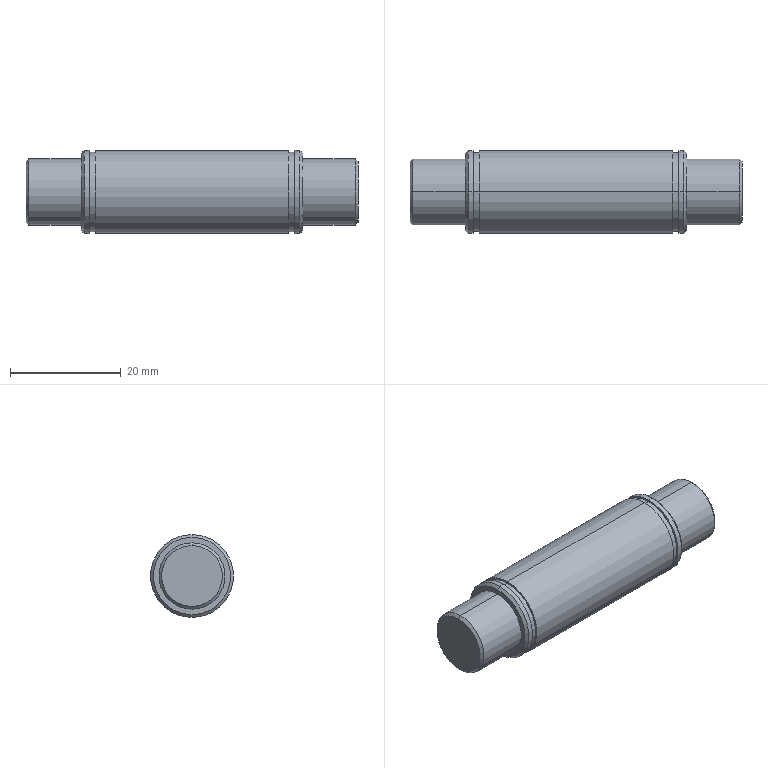Part | SolidWorks | features MirrorPattern 2, Chamfer 1, Extrusion 1, ICE 1, RevCut 1 | 1 solid | 30 faces | box 60 x 15 x 15 mm | volume 9274 mm3 | cylinder 14 | cone 8 | plane 8 | commonest cylinder face diameters 15 x6 12 x4 14.3 x4
STEP:
#1=CARTESIAN_POINT('',(19.5,0.,7.5));
#2=VERTEX_POINT('',#1);
#3=CARTESIAN_POINT('',(19.5,0.,-7.5));
#4=VERTEX_POINT('',#3);
#5=CARTESIAN_POINT('',(19.5,0.,0.));
#6=DIRECTION('',(-1.,0.,0.));
#7=DIRECTION('',(0.,0.,-1.));
#8=AXIS2_PLACEMENT_3D('',#5,#6,#7);
#9=CIRCLE('',#8,7.5);
#10=EDGE_CURVE('',#2,#4,#9,.T.);
#11=ORIENTED_EDGE('',*,*,#10,.T.);
#12=CARTESIAN_POINT('',(18.6,0.,-7.5));
#13=VERTEX_POINT('',#12);
#14=CARTESIAN_POINT('',(30.,0.,-7.5));
#15=DIRECTION('',(-1.,0.,0.));
#16=VECTOR('',#15,1000.);
#17=LINE('',#14,#16);
#18=EDGE_CURVE('',#4,#13,#17,.T.);
#19=ORIENTED_EDGE('',*,*,#18,.T.);
#20=CARTESIAN_POINT('',(18.6,0.,7.5));
#21=VERTEX_POINT('',#20);
#22=CARTESIAN_POINT('',(18.6,0.,0.));
#23=DIRECTION('',(-1.,0.,0.));
#24=DIRECTION('',(0.,0.,1.));
#25=AXIS2_PLACEMENT_3D('',#22,#23,#24);
#26=CIRCLE('',#25,7.5);
#27=EDGE_CURVE('',#21,#13,#26,.T.);
#28=ORIENTED_EDGE('',*,*,#27,.F.);
#29=CARTESIAN_POINT('',(30.,0.,7.5));
#30=DIRECTION('',(-1.,0.,0.));
#31=VECTOR('',#30,1000.);
#32=LINE('',#29,#31);
#33=EDGE_CURVE('',#2,#21,#32,.T.);
#34=ORIENTED_EDGE('',*,*,#33,.F.);
#35=EDGE_LOOP('',(#11,#19,#28,#34));
#36=FACE_OUTER_BOUND('',#35,.T.);
#37=CARTESIAN_POINT('',(30.,0.,0.));
#38=DIRECTION('',(-1.,0.,0.));
#39=DIRECTION('',(0.,0.,1.));
#40=AXIS2_PLACEMENT_3D('',#37,#38,#39);
#41=CYLINDRICAL_SURFACE('',#40,7.5);
#42=ADVANCED_FACE('',(#36),#41,.T.);
#43=CARTESIAN_POINT('',(20.,0.,-7.));
#44=VERTEX_POINT('',#43);
#45=CARTESIAN_POINT('',(20.,0.,7.));
#46=VERTEX_POINT('',#45);
#47=CARTESIAN_POINT('',(20.,0.,0.));
#48=DIRECTION('',(1.,0.,0.));
#49=DIRECTION('',(0.,0.,-1.));
#50=AXIS2_PLACEMENT_3D('',#47,#48,#49);
#51=CIRCLE('',#50,7.);
#52=EDGE_CURVE('',#44,#46,#51,.T.);
#53=ORIENTED_EDGE('',*,*,#52,.F.);
#54=CARTESIAN_POINT('',(20.,0.,-7.));
#55=DIRECTION('',(-0.7071,0.,-0.7071));
#56=VECTOR('',#55,1000.);
#57=LINE('',#54,#56);
#58=EDGE_CURVE('',#44,#4,#57,.T.);
#59=ORIENTED_EDGE('',*,*,#58,.T.);
#60=ORIENTED_EDGE('',*,*,#10,.F.);
#61=CARTESIAN_POINT('',(20.,0.,7.));
#62=DIRECTION('',(-0.7071,0.,0.7071));
#63=VECTOR('',#62,1000.);
#64=LINE('',#61,#63);
#65=EDGE_CURVE('',#46,#2,#64,.T.);
#66=ORIENTED_EDGE('',*,*,#65,.F.);
#67=EDGE_LOOP('',(#53,#59,#60,#66));
#68=FACE_OUTER_BOUND('',#67,.T.);
#69=CARTESIAN_POINT('',(20.,0.,0.));
#70=DIRECTION('',(-1.,0.,0.));
#71=DIRECTION('',(0.,0.,1.));
#72=AXIS2_PLACEMENT_3D('',#69,#70,#71);
#73=CONICAL_SURFACE('',#72,7.,0.7854);
#74=ADVANCED_FACE('',(#68),#73,.T.);
#75=CARTESIAN_POINT('',(20.,0.,-6.));
#76=VERTEX_POINT('',#75);
#77=CARTESIAN_POINT('',(20.,0.,6.));
#78=VERTEX_POINT('',#77);
#79=CARTESIAN_POINT('',(20.,0.,0.));
#80=DIRECTION('',(1.,0.,0.));
#81=DIRECTION('',(0.,0.,-1.));
#82=AXIS2_PLACEMENT_3D('',#79,#80,#81);
#83=CIRCLE('',#82,6.);
#84=EDGE_CURVE('',#76,#78,#83,.T.);
#85=ORIENTED_EDGE('',*,*,#84,.T.);
#86=CARTESIAN_POINT('',(29.5,0.,6.));
#87=VERTEX_POINT('',#86);
#88=CARTESIAN_POINT('',(20.,0.,6.));
#89=DIRECTION('',(1.,0.,0.));
#90=VECTOR('',#89,1000.);
#91=LINE('',#88,#90);
#92=EDGE_CURVE('',#78,#87,#91,.T.);
#93=ORIENTED_EDGE('',*,*,#92,.T.);
#94=CARTESIAN_POINT('',(29.5,0.,-6.));
#95=VERTEX_POINT('',#94);
#96=CARTESIAN_POINT('',(29.5,0.,0.));
#97=DIRECTION('',(-1.,0.,0.));
#98=DIRECTION('',(0.,0.,-1.));
#99=AXIS2_PLACEMENT_3D('',#96,#97,#98);
#100=CIRCLE('',#99,6.);
#101=EDGE_CURVE('',#87,#95,#100,.T.);
#102=ORIENTED_EDGE('',*,*,#101,.T.);
#103=CARTESIAN_POINT('',(20.,0.,-6.));
#104=DIRECTION('',(1.,0.,0.));
#105=VECTOR('',#104,1000.);
#106=LINE('',#103,#105);
#107=EDGE_CURVE('',#76,#95,#106,.T.);
#108=ORIENTED_EDGE('',*,*,#107,.F.);
#109=EDGE_LOOP('',(#85,#93,#102,#108));
#110=FACE_OUTER_BOUND('',#109,.T.);
#111=CARTESIAN_POINT('',(20.,0.,0.));
#112=DIRECTION('',(1.,0.,0.));
#113=DIRECTION('',(0.,0.,-1.));
#114=AXIS2_PLACEMENT_3D('',#111,#112,#113);
#115=CYLINDRICAL_SURFACE('',#114,6.);
#116=ADVANCED_FACE('',(#110),#115,.T.);
#117=CARTESIAN_POINT('',(30.,0.,-5.5));
#118=VERTEX_POINT('',#117);
#119=CARTESIAN_POINT('',(30.,0.,5.5));
#120=VERTEX_POINT('',#119);
#121=CARTESIAN_POINT('',(30.,0.,0.));
#122=DIRECTION('',(1.,0.,0.));
#123=DIRECTION('',(0.,0.,-1.));
#124=AXIS2_PLACEMENT_3D('',#121,#122,#123);
#125=CIRCLE('',#124,5.5);
#126=EDGE_CURVE('',#118,#120,#125,.T.);
#127=ORIENTED_EDGE('',*,*,#126,.F.);
#128=CARTESIAN_POINT('',(30.,0.,-5.5));
#129=DIRECTION('',(-0.7071,0.,-0.7071));
#130=VECTOR('',#129,1000.);
#131=LINE('',#128,#130);
#132=EDGE_CURVE('',#118,#95,#131,.T.);
#133=ORIENTED_EDGE('',*,*,#132,.T.);
#134=ORIENTED_EDGE('',*,*,#101,.F.);
#135=CARTESIAN_POINT('',(30.,0.,5.5));
#136=DIRECTION('',(-0.7071,0.,0.7071));
#137=VECTOR('',#136,1000.);
#138=LINE('',#135,#137);
#139=EDGE_CURVE('',#120,#87,#138,.T.);
#140=ORIENTED_EDGE('',*,*,#139,.F.);
#141=EDGE_LOOP('',(#127,#133,#134,#140));
#142=FACE_OUTER_BOUND('',#141,.T.);
#143=CARTESIAN_POINT('',(30.,0.,0.));
#144=DIRECTION('',(-1.,0.,0.));
#145=DIRECTION('',(0.,0.,1.));
#146=AXIS2_PLACEMENT_3D('',#143,#144,#145);
#147=CONICAL_SURFACE('',#146,5.5,0.7854);
#148=ADVANCED_FACE('',(#142),#147,.T.);
#149=CARTESIAN_POINT('',(17.5,0.,-7.15));
#150=VERTEX_POINT('',#149);
#151=CARTESIAN_POINT('',(17.5,0.,7.15));
#152=VERTEX_POINT('',#151);
#153=CARTESIAN_POINT('',(17.5,0.,0.));
#154=DIRECTION('',(-1.,0.,0.));
#155=DIRECTION('',(0.,0.,1.));
#156=AXIS2_PLACEMENT_3D('',#153,#154,#155);
#157=CIRCLE('',#156,7.15);
#158=EDGE_CURVE('',#150,#152,#157,.T.);
#159=ORIENTED_EDGE('',*,*,#158,.F.);
#160=CARTESIAN_POINT('',(18.6,0.,-7.15));
#161=VERTEX_POINT('',#160);
#162=CARTESIAN_POINT('',(31.366,0.,-7.15));
#163=DIRECTION('',(1.,0.,0.));
#164=VECTOR('',#163,1000.);
#165=LINE('',#162,#164);
#166=EDGE_CURVE('',#150,#161,#165,.T.);
#167=ORIENTED_EDGE('',*,*,#166,.T.);
#168=CARTESIAN_POINT('',(18.6,0.,7.15));
#169=VERTEX_POINT('',#168);
#170=CARTESIAN_POINT('',(18.6,0.,0.));
#171=DIRECTION('',(-1.,0.,0.));
#172=DIRECTION('',(0.,0.,1.));
#173=AXIS2_PLACEMENT_3D('',#170,#171,#172);
#174=CIRCLE('',#173,7.15);
#175=EDGE_CURVE('',#161,#169,#174,.T.);
#176=ORIENTED_EDGE('',*,*,#175,.T.);
#177=CARTESIAN_POINT('',(31.366,0.,7.15));
#178=DIRECTION('',(1.,0.,0.));
#179=VECTOR('',#178,1000.);
#180=LINE('',#177,#179);
#181=EDGE_CURVE('',#152,#169,#180,.T.);
#182=ORIENTED_EDGE('',*,*,#181,.F.);
#183=EDGE_LOOP('',(#159,#167,#176,#182));
#184=FACE_OUTER_BOUND('',#183,.T.);
#185=CARTESIAN_POINT('',(31.366,0.,0.));
#186=DIRECTION('',(1.,0.,0.));
#187=DIRECTION('',(0.,0.,1.));
#188=AXIS2_PLACEMENT_3D('',#185,#186,#187);
#189=CYLINDRICAL_SURFACE('',#188,7.15);
#190=ADVANCED_FACE('',(#184),#189,.T.);
#191=CARTESIAN_POINT('',(17.5,0.,7.5));
#192=VERTEX_POINT('',#191);
#193=CARTESIAN_POINT('',(17.5,0.,-7.5));
#194=VERTEX_POINT('',#193);
#195=CARTESIAN_POINT('',(17.5,0.,0.));
#196=DIRECTION('',(-1.,0.,0.));
#197=DIRECTION('',(0.,0.,1.));
#198=AXIS2_PLACEMENT_3D('',#195,#196,#197);
#199=CIRCLE('',#198,7.5);
#200=EDGE_CURVE('',#192,#194,#199,.T.);
#201=ORIENTED_EDGE('',*,*,#200,.T.);
#202=CARTESIAN_POINT('',(-17.5,0.,-7.5));
#203=VERTEX_POINT('',#202);
#204=CARTESIAN_POINT('',(30.,0.,-7.5));
#205=DIRECTION('',(-1.,0.,0.));
#206=VECTOR('',#205,1000.);
#207=LINE('',#204,#206);
#208=EDGE_CURVE('',#194,#203,#207,.T.);
#209=ORIENTED_EDGE('',*,*,#208,.T.);
#210=CARTESIAN_POINT('',(-17.5,0.,7.5));
#211=VERTEX_POINT('',#210);
#212=CARTESIAN_POINT('',(-17.5,0.,0.));
#213=DIRECTION('',(-1.,0.,0.));
#214=DIRECTION('',(0.,0.,1.));
#215=AXIS2_PLACEMENT_3D('',#212,#213,#214);
#216=CIRCLE('',#215,7.5);
#217=EDGE_CURVE('',#211,#203,#216,.T.);
#218=ORIENTED_EDGE('',*,*,#217,.F.);
#219=CARTESIAN_POINT('',(30.,0.,7.5));
#220=DIRECTION('',(-1.,0.,0.));
#221=VECTOR('',#220,1000.);
#222=LINE('',#219,#221);
#223=EDGE_CURVE('',#192,#211,#222,.T.);
#224=ORIENTED_EDGE('',*,*,#223,.F.);
#225=EDGE_LOOP('',(#201,#209,#218,#224));
#226=FACE_OUTER_BOUND('',#225,.T.);
#227=CARTESIAN_POINT('',(30.,0.,0.));
#228=DIRECTION('',(-1.,0.,0.));
#229=DIRECTION('',(0.,0.,1.));
#230=AXIS2_PLACEMENT_3D('',#227,#228,#229);
#231=CYLINDRICAL_SURFACE('',#230,7.5);
#232=ADVANCED_FACE('',(#226),#231,.T.);
#233=CARTESIAN_POINT('',(-17.5,0.,7.15));
#234=VERTEX_POINT('',#233);
#235=CARTESIAN_POINT('',(-17.5,0.,-7.15));
#236=VERTEX_POINT('',#235);
#237=CARTESIAN_POINT('',(-17.5,0.,0.));
#238=DIRECTION('',(-1.,0.,0.));
#239=DIRECTION('',(0.,0.,1.));
#240=AXIS2_PLACEMENT_3D('',#237,#238,#239);
#241=CIRCLE('',#240,7.15);
#242=EDGE_CURVE('',#234,#236,#241,.T.);
#243=ORIENTED_EDGE('',*,*,#242,.T.);
#244=CARTESIAN_POINT('',(-18.6,0.,-7.15));
#245=VERTEX_POINT('',#244);
#246=CARTESIAN_POINT('',(-31.366,0.,-7.15));
#247=DIRECTION('',(-1.,0.,0.));
#248=VECTOR('',#247,1000.);
#249=LINE('',#246,#248);
#250=EDGE_CURVE('',#236,#245,#249,.T.);
#251=ORIENTED_EDGE('',*,*,#250,.T.);
#252=CARTESIAN_POINT('',(-18.6,0.,7.15));
#253=VERTEX_POINT('',#252);
#254=CARTESIAN_POINT('',(-18.6,0.,0.));
#255=DIRECTION('',(-1.,0.,0.));
#256=DIRECTION('',(0.,0.,1.));
#257=AXIS2_PLACEMENT_3D('',#254,#255,#256);
#258=CIRCLE('',#257,7.15);
#259=EDGE_CURVE('',#253,#245,#258,.T.);
#260=ORIENTED_EDGE('',*,*,#259,.F.);
#261=CARTESIAN_POINT('',(-31.366,0.,7.15));
#262=DIRECTION('',(-1.,0.,0.));
#263=VECTOR('',#262,1000.);
#264=LINE('',#261,#263);
#265=EDGE_CURVE('',#234,#253,#264,.T.);
#266=ORIENTED_EDGE('',*,*,#265,.F.);
#267=EDGE_LOOP('',(#243,#251,#260,#266));
#268=FACE_OUTER_BOUND('',#267,.T.);
#269=CARTESIAN_POINT('',(-31.366,0.,0.));
#270=DIRECTION('',(-1.,0.,0.));
#271=DIRECTION('',(0.,0.,1.));
#272=AXIS2_PLACEMENT_3D('',#269,#270,#271);
#273=CYLINDRICAL_SURFACE('',#272,7.15);
#274=ADVANCED_FACE('',(#268),#273,.T.);
#275=CARTESIAN_POINT('',(-30.,0.,5.5));
#276=VERTEX_POINT('',#275);
#277=CARTESIAN_POINT('',(-30.,0.,-5.5));
#278=VERTEX_POINT('',#277);
#279=CARTESIAN_POINT('',(-30.,0.,0.));
#280=DIRECTION('',(-1.,0.,0.));
#281=DIRECTION('',(0.,0.,-1.));
#282=AXIS2_PLACEMENT_3D('',#279,#280,#281);
#283=CIRCLE('',#282,5.5);
#284=EDGE_CURVE('',#276,#278,#283,.T.);
#285=ORIENTED_EDGE('',*,*,#284,.F.);
#286=CARTESIAN_POINT('',(-29.5,0.,6.));
#287=VERTEX_POINT('',#286);
#288=CARTESIAN_POINT('',(-29.5,0.,6.));
#289=DIRECTION('',(0.7071,0.,0.7071));
#290=VECTOR('',#289,1000.);
#291=LINE('',#288,#290);
#292=EDGE_CURVE('',#276,#287,#291,.T.);
#293=ORIENTED_EDGE('',*,*,#292,.T.);
#294=CARTESIAN_POINT('',(-29.5,0.,-6.));
#295=VERTEX_POINT('',#294);
#296=CARTESIAN_POINT('',(-29.5,0.,0.));
#297=DIRECTION('',(1.,0.,0.));
#298=DIRECTION('',(0.,0.,-1.));
#299=AXIS2_PLACEMENT_3D('',#296,#297,#298);
#300=CIRCLE('',#299,6.);
#301=EDGE_CURVE('',#295,#287,#300,.T.);
#302=ORIENTED_EDGE('',*,*,#301,.F.);
#303=CARTESIAN_POINT('',(-29.5,0.,-6.));
#304=DIRECTION('',(0.7071,0.,-0.7071));
#305=VECTOR('',#304,1000.);
#306=LINE('',#303,#305);
#307=EDGE_CURVE('',#278,#295,#306,.T.);
#308=ORIENTED_EDGE('',*,*,#307,.F.);
#309=EDGE_LOOP('',(#285,#293,#302,#308));
#310=FACE_OUTER_BOUND('',#309,.T.);
#311=CARTESIAN_POINT('',(-29.5,0.,0.));
#312=DIRECTION('',(1.,0.,0.));
#313=DIRECTION('',(0.,0.,-1.));
#314=AXIS2_PLACEMENT_3D('',#311,#312,#313);
#315=CONICAL_SURFACE('',#314,6.,0.7854);
#316=ADVANCED_FACE('',(#310),#315,.T.);
#317=CARTESIAN_POINT('',(-20.,0.,7.));
#318=VERTEX_POINT('',#317);
#319=CARTESIAN_POINT('',(-20.,0.,-7.));
#320=VERTEX_POINT('',#319);
#321=CARTESIAN_POINT('',(-20.,0.,0.));
#322=DIRECTION('',(-1.,0.,0.));
#323=DIRECTION('',(0.,0.,1.));
#324=AXIS2_PLACEMENT_3D('',#321,#322,#323);
#325=CIRCLE('',#324,7.);
#326=EDGE_CURVE('',#318,#320,#325,.T.);
#327=ORIENTED_EDGE('',*,*,#326,.F.);
#328=CARTESIAN_POINT('',(-19.5,0.,7.5));
#329=VERTEX_POINT('',#328);
#330=CARTESIAN_POINT('',(-20.,0.,7.));
#331=DIRECTION('',(0.7071,0.,0.7071));
#332=VECTOR('',#331,1000.);
#333=LINE('',#330,#332);
#334=EDGE_CURVE('',#318,#329,#333,.T.);
#335=ORIENTED_EDGE('',*,*,#334,.T.);
#336=CARTESIAN_POINT('',(-19.5,0.,-7.5));
#337=VERTEX_POINT('',#336);
#338=CARTESIAN_POINT('',(-19.5,0.,0.));
#339=DIRECTION('',(1.,0.,0.));
#340=DIRECTION('',(0.,0.,1.));
#341=AXIS2_PLACEMENT_3D('',#338,#339,#340);
#342=CIRCLE('',#341,7.5);
#343=EDGE_CURVE('',#337,#329,#342,.T.);
#344=ORIENTED_EDGE('',*,*,#343,.F.);
#345=CARTESIAN_POINT('',(-20.,0.,-7.));
#346=DIRECTION('',(0.7071,0.,-0.7071));
#347=VECTOR('',#346,1000.);
#348=LINE('',#345,#347);
#349=EDGE_CURVE('',#320,#337,#348,.T.);
#350=ORIENTED_EDGE('',*,*,#349,.F.);
#351=EDGE_LOOP('',(#327,#335,#344,#350));
#352=FACE_OUTER_BOUND('',#351,.T.);
#353=CARTESIAN_POINT('',(-20.,0.,0.));
#354=DIRECTION('',(1.,0.,0.));
#355=DIRECTION('',(0.,0.,-1.));
#356=AXIS2_PLACEMENT_3D('',#353,#354,#355);
#357=CONICAL_SURFACE('',#356,7.,0.7854);
#358=ADVANCED_FACE('',(#352),#357,.T.);
#359=CARTESIAN_POINT('',(-20.,0.,-6.));
#360=VERTEX_POINT('',#359);
#361=CARTESIAN_POINT('',(-20.,0.,6.));
#362=VERTEX_POINT('',#361);
#363=CARTESIAN_POINT('',(-20.,0.,0.));
#364=DIRECTION('',(1.,0.,0.));
#365=DIRECTION('',(0.,0.,-1.));
#366=AXIS2_PLACEMENT_3D('',#363,#364,#365);
#367=CIRCLE('',#366,6.);
#368=EDGE_CURVE('',#360,#362,#367,.T.);
#369=ORIENTED_EDGE('',*,*,#368,.F.);
#370=CARTESIAN_POINT('',(-20.,0.,-6.));
#371=DIRECTION('',(-1.,0.,0.));
#372=VECTOR('',#371,1000.);
#373=LINE('',#370,#372);
#374=EDGE_CURVE('',#360,#295,#373,.T.);
#375=ORIENTED_EDGE('',*,*,#374,.T.);
#376=ORIENTED_EDGE('',*,*,#301,.T.);
#377=CARTESIAN_POINT('',(-20.,0.,6.));
#378=DIRECTION('',(-1.,0.,0.));
#379=VECTOR('',#378,1000.);
#380=LINE('',#377,#379);
#381=EDGE_CURVE('',#362,#287,#380,.T.);
#382=ORIENTED_EDGE('',*,*,#381,.F.);
#383=EDGE_LOOP('',(#369,#375,#376,#382));
#384=FACE_OUTER_BOUND('',#383,.T.);
#385=CARTESIAN_POINT('',(-20.,0.,0.));
#386=DIRECTION('',(-1.,0.,0.));
#387=DIRECTION('',(0.,0.,1.));
#388=AXIS2_PLACEMENT_3D('',#385,#386,#387);
#389=CYLINDRICAL_SURFACE('',#388,6.);
#390=ADVANCED_FACE('',(#384),#389,.T.);
#391=CARTESIAN_POINT('',(-18.6,0.,7.5));
#392=VERTEX_POINT('',#391);
#393=CARTESIAN_POINT('',(-18.6,0.,-7.5));
#394=VERTEX_POINT('',#393);
#395=CARTESIAN_POINT('',(-18.6,0.,0.));
#396=DIRECTION('',(-1.,0.,0.));
#397=DIRECTION('',(0.,0.,1.));
#398=AXIS2_PLACEMENT_3D('',#395,#396,#397);
#399=CIRCLE('',#398,7.5);
#400=EDGE_CURVE('',#392,#394,#399,.T.);
#401=ORIENTED_EDGE('',*,*,#400,.T.);
#402=CARTESIAN_POINT('',(30.,0.,-7.5));
#403=DIRECTION('',(-1.,0.,0.));
#404=VECTOR('',#403,1000.);
#405=LINE('',#402,#404);
#406=EDGE_CURVE('',#394,#337,#405,.T.);
#407=ORIENTED_EDGE('',*,*,#406,.T.);
#408=ORIENTED_EDGE('',*,*,#343,.T.);
#409=CARTESIAN_POINT('',(30.,0.,7.5));
#410=DIRECTION('',(-1.,0.,0.));
#411=VECTOR('',#410,1000.);
#412=LINE('',#409,#411);
#413=EDGE_CURVE('',#392,#329,#412,.T.);
#414=ORIENTED_EDGE('',*,*,#413,.F.);
#415=EDGE_LOOP('',(#401,#407,#408,#414));
#416=FACE_OUTER_BOUND('',#415,.T.);
#417=CARTESIAN_POINT('',(30.,0.,0.));
#418=DIRECTION('',(-1.,0.,0.));
#419=DIRECTION('',(0.,0.,1.));
#420=AXIS2_PLACEMENT_3D('',#417,#418,#419);
#421=CYLINDRICAL_SURFACE('',#420,7.5);
#422=ADVANCED_FACE('',(#416),#421,.T.);
#423=ORIENTED_EDGE('',*,*,#406,.F.);
#424=CARTESIAN_POINT('',(-18.6,0.,0.));
#425=DIRECTION('',(-1.,0.,0.));
#426=DIRECTION('',(0.,0.,1.));
#427=AXIS2_PLACEMENT_3D('',#424,#425,#426);
#428=CIRCLE('',#427,7.5);
#429=EDGE_CURVE('',#394,#392,#428,.T.);
#430=ORIENTED_EDGE('',*,*,#429,.T.);
#431=ORIENTED_EDGE('',*,*,#413,.T.);
#432=CARTESIAN_POINT('',(-19.5,0.,0.));
#433=DIRECTION('',(1.,0.,0.));
#434=DIRECTION('',(0.,0.,1.));
#435=AXIS2_PLACEMENT_3D('',#432,#433,#434);
#436=CIRCLE('',#435,7.5);
#437=EDGE_CURVE('',#329,#337,#436,.T.);
#438=ORIENTED_EDGE('',*,*,#437,.T.);
#439=EDGE_LOOP('',(#423,#430,#431,#438));
#440=FACE_OUTER_BOUND('',#439,.T.);
#441=CARTESIAN_POINT('',(30.,0.,0.));
#442=DIRECTION('',(-1.,0.,0.));
#443=DIRECTION('',(0.,0.,1.));
#444=AXIS2_PLACEMENT_3D('',#441,#442,#443);
#445=CYLINDRICAL_SURFACE('',#444,7.5);
#446=ADVANCED_FACE('',(#440),#445,.T.);
#447=CARTESIAN_POINT('',(-20.,0.,0.));
#448=DIRECTION('',(-1.,0.,0.));
#449=DIRECTION('',(0.,0.,1.));
#450=AXIS2_PLACEMENT_3D('',#447,#448,#449);
#451=CIRCLE('',#450,7.);
#452=EDGE_CURVE('',#320,#318,#451,.T.);
#453=ORIENTED_EDGE('',*,*,#452,.T.);
#454=ORIENTED_EDGE('',*,*,#326,.T.);
#455=EDGE_LOOP('',(#453,#454));
#456=FACE_OUTER_BOUND('',#455,.T.);
#457=CARTESIAN_POINT('',(-20.,0.,0.));
#458=DIRECTION('',(1.,0.,0.));
#459=DIRECTION('',(0.,0.,-1.));
#460=AXIS2_PLACEMENT_3D('',#457,#458,#459);
#461=CIRCLE('',#460,6.);
#462=EDGE_CURVE('',#362,#360,#461,.T.);
#463=ORIENTED_EDGE('',*,*,#462,.T.);
#464=ORIENTED_EDGE('',*,*,#368,.T.);
#465=EDGE_LOOP('',(#463,#464));
#466=FACE_BOUND('',#465,.T.);
#467=CARTESIAN_POINT('',(-20.,0.,0.));
#468=DIRECTION('',(-1.,0.,0.));
#469=DIRECTION('',(0.,0.,1.));
#470=AXIS2_PLACEMENT_3D('',#467,#468,#469);
#471=PLANE('',#470);
#472=ADVANCED_FACE('',(#456,#466),#471,.T.);
#473=ORIENTED_EDGE('',*,*,#374,.F.);
#474=ORIENTED_EDGE('',*,*,#462,.F.);
#475=ORIENTED_EDGE('',*,*,#381,.T.);
#476=CARTESIAN_POINT('',(-29.5,0.,0.));
#477=DIRECTION('',(1.,0.,0.));
#478=DIRECTION('',(0.,0.,-1.));
#479=AXIS2_PLACEMENT_3D('',#476,#477,#478);
#480=CIRCLE('',#479,6.);
#481=EDGE_CURVE('',#287,#295,#480,.T.);
#482=ORIENTED_EDGE('',*,*,#481,.T.);
#483=EDGE_LOOP('',(#473,#474,#475,#482));
#484=FACE_OUTER_BOUND('',#483,.T.);
#485=CARTESIAN_POINT('',(-20.,0.,0.));
#486=DIRECTION('',(-1.,0.,0.));
#487=DIRECTION('',(0.,0.,1.));
#488=AXIS2_PLACEMENT_3D('',#485,#486,#487);
#489=CYLINDRICAL_SURFACE('',#488,6.);
#490=ADVANCED_FACE('',(#484),#489,.T.);
#491=CARTESIAN_POINT('',(-30.,0.,0.));
#492=DIRECTION('',(-1.,0.,0.));
#493=DIRECTION('',(0.,0.,-1.));
#494=AXIS2_PLACEMENT_3D('',#491,#492,#493);
#495=CIRCLE('',#494,5.5);
#496=EDGE_CURVE('',#278,#276,#495,.T.);
#497=ORIENTED_EDGE('',*,*,#496,.T.);
#498=ORIENTED_EDGE('',*,*,#284,.T.);
#499=EDGE_LOOP('',(#497,#498));
#500=FACE_OUTER_BOUND('',#499,.T.);
#501=CARTESIAN_POINT('',(-30.,0.,0.));
#502=DIRECTION('',(1.,0.,0.));
#503=DIRECTION('',(0.,0.,-1.));
#504=AXIS2_PLACEMENT_3D('',#501,#502,#503);
#505=PLANE('',#504);
#506=ADVANCED_FACE('',(#500),#505,.F.);
#507=ORIENTED_EDGE('',*,*,#334,.F.);
#508=ORIENTED_EDGE('',*,*,#452,.F.);
#509=ORIENTED_EDGE('',*,*,#349,.T.);
#510=ORIENTED_EDGE('',*,*,#437,.F.);
#511=EDGE_LOOP('',(#507,#508,#509,#510));
#512=FACE_OUTER_BOUND('',#511,.T.);
#513=CARTESIAN_POINT('',(-20.,0.,0.));
#514=DIRECTION('',(1.,0.,0.));
#515=DIRECTION('',(0.,0.,-1.));
#516=AXIS2_PLACEMENT_3D('',#513,#514,#515);
#517=CONICAL_SURFACE('',#516,7.,0.7854);
#518=ADVANCED_FACE('',(#512),#517,.T.);
#519=ORIENTED_EDGE('',*,*,#292,.F.);
#520=ORIENTED_EDGE('',*,*,#496,.F.);
#521=ORIENTED_EDGE('',*,*,#307,.T.);
#522=ORIENTED_EDGE('',*,*,#481,.F.);
#523=EDGE_LOOP('',(#519,#520,#521,#522));
#524=FACE_OUTER_BOUND('',#523,.T.);
#525=CARTESIAN_POINT('',(-29.5,0.,0.));
#526=DIRECTION('',(1.,0.,0.));
#527=DIRECTION('',(0.,0.,-1.));
#528=AXIS2_PLACEMENT_3D('',#525,#526,#527);
#529=CONICAL_SURFACE('',#528,6.,0.7854);
#530=ADVANCED_FACE('',(#524),#529,.T.);
#531=ORIENTED_EDGE('',*,*,#400,.F.);
#532=ORIENTED_EDGE('',*,*,#429,.F.);
#533=EDGE_LOOP('',(#531,#532));
#534=FACE_OUTER_BOUND('',#533,.T.);
#535=ORIENTED_EDGE('',*,*,#259,.T.);
#536=CARTESIAN_POINT('',(-18.6,0.,0.));
#537=DIRECTION('',(-1.,0.,0.));
#538=DIRECTION('',(0.,0.,1.));
#539=AXIS2_PLACEMENT_3D('',#536,#537,#538);
#540=CIRCLE('',#539,7.15);
#541=EDGE_CURVE('',#245,#253,#540,.T.);
#542=ORIENTED_EDGE('',*,*,#541,.T.);
#543=EDGE_LOOP('',(#535,#542));
#544=FACE_BOUND('',#543,.T.);
#545=CARTESIAN_POINT('',(-18.6,-7.5,0.));
#546=DIRECTION('',(-1.,0.,0.));
#547=DIRECTION('',(0.,0.,1.));
#548=AXIS2_PLACEMENT_3D('',#545,#546,#547);
#549=PLANE('',#548);
#550=ADVANCED_FACE('',(#534,#544),#549,.F.);
#551=ORIENTED_EDGE('',*,*,#250,.F.);
#552=CARTESIAN_POINT('',(-17.5,0.,0.));
#553=DIRECTION('',(-1.,0.,0.));
#554=DIRECTION('',(0.,0.,1.));
#555=AXIS2_PLACEMENT_3D('',#552,#553,#554);
#556=CIRCLE('',#555,7.15);
#557=EDGE_CURVE('',#236,#234,#556,.T.);
#558=ORIENTED_EDGE('',*,*,#557,.T.);
#559=ORIENTED_EDGE('',*,*,#265,.T.);
#560=ORIENTED_EDGE('',*,*,#541,.F.);
#561=EDGE_LOOP('',(#551,#558,#559,#560));
#562=FACE_OUTER_BOUND('',#561,.T.);
#563=CARTESIAN_POINT('',(-31.366,0.,0.));
#564=DIRECTION('',(-1.,0.,0.));
#565=DIRECTION('',(0.,0.,1.));
#566=AXIS2_PLACEMENT_3D('',#563,#564,#565);
#567=CYLINDRICAL_SURFACE('',#566,7.15);
#568=ADVANCED_FACE('',(#562),#567,.T.);
#569=ORIENTED_EDGE('',*,*,#242,.F.);
#570=ORIENTED_EDGE('',*,*,#557,.F.);
#571=EDGE_LOOP('',(#569,#570));
#572=FACE_BOUND('',#571,.T.);
#573=ORIENTED_EDGE('',*,*,#217,.T.);
#574=CARTESIAN_POINT('',(-17.5,0.,0.));
#575=DIRECTION('',(-1.,0.,0.));
#576=DIRECTION('',(0.,0.,1.));
#577=AXIS2_PLACEMENT_3D('',#574,#575,#576);
#578=CIRCLE('',#577,7.5);
#579=EDGE_CURVE('',#203,#211,#578,.T.);
#580=ORIENTED_EDGE('',*,*,#579,.T.);
#581=EDGE_LOOP('',(#573,#580));
#582=FACE_OUTER_BOUND('',#581,.T.);
#583=CARTESIAN_POINT('',(-17.5,-7.5,0.));
#584=DIRECTION('',(1.,0.,0.));
#585=DIRECTION('',(0.,0.,-1.));
#586=AXIS2_PLACEMENT_3D('',#583,#584,#585);
#587=PLANE('',#586);
#588=ADVANCED_FACE('',(#572,#582),#587,.F.);
#589=ORIENTED_EDGE('',*,*,#208,.F.);
#590=CARTESIAN_POINT('',(17.5,0.,0.));
#591=DIRECTION('',(-1.,0.,0.));
#592=DIRECTION('',(0.,0.,1.));
#593=AXIS2_PLACEMENT_3D('',#590,#591,#592);
#594=CIRCLE('',#593,7.5);
#595=EDGE_CURVE('',#194,#192,#594,.T.);
#596=ORIENTED_EDGE('',*,*,#595,.T.);
#597=ORIENTED_EDGE('',*,*,#223,.T.);
#598=ORIENTED_EDGE('',*,*,#579,.F.);
#599=EDGE_LOOP('',(#589,#596,#597,#598));
#600=FACE_OUTER_BOUND('',#599,.T.);
#601=CARTESIAN_POINT('',(30.,0.,0.));
#602=DIRECTION('',(-1.,0.,0.));
#603=DIRECTION('',(0.,0.,1.));
#604=AXIS2_PLACEMENT_3D('',#601,#602,#603);
#605=CYLINDRICAL_SURFACE('',#604,7.5);
#606=ADVANCED_FACE('',(#600),#605,.T.);
#607=ORIENTED_EDGE('',*,*,#27,.T.);
#608=CARTESIAN_POINT('',(18.6,0.,0.));
#609=DIRECTION('',(-1.,0.,0.));
#610=DIRECTION('',(0.,0.,1.));
#611=AXIS2_PLACEMENT_3D('',#608,#609,#610);
#612=CIRCLE('',#611,7.5);
#613=EDGE_CURVE('',#13,#21,#612,.T.);
#614=ORIENTED_EDGE('',*,*,#613,.T.);
#615=EDGE_LOOP('',(#607,#614));
#616=FACE_OUTER_BOUND('',#615,.T.);
#617=CARTESIAN_POINT('',(18.6,0.,0.));
#618=DIRECTION('',(-1.,0.,0.));
#619=DIRECTION('',(0.,0.,1.));
#620=AXIS2_PLACEMENT_3D('',#617,#618,#619);
#621=CIRCLE('',#620,7.15);
#622=EDGE_CURVE('',#169,#161,#621,.T.);
#623=ORIENTED_EDGE('',*,*,#622,.F.);
#624=ORIENTED_EDGE('',*,*,#175,.F.);
#625=EDGE_LOOP('',(#623,#624));
#626=FACE_BOUND('',#625,.T.);
#627=CARTESIAN_POINT('',(18.6,-7.5,0.));
#628=DIRECTION('',(1.,0.,0.));
#629=DIRECTION('',(0.,0.,1.));
#630=AXIS2_PLACEMENT_3D('',#627,#628,#629);
#631=PLANE('',#630);
#632=ADVANCED_FACE('',(#616,#626),#631,.F.);
#633=ORIENTED_EDGE('',*,*,#166,.F.);
#634=CARTESIAN_POINT('',(17.5,0.,0.));
#635=DIRECTION('',(-1.,0.,0.));
#636=DIRECTION('',(0.,0.,1.));
#637=AXIS2_PLACEMENT_3D('',#634,#635,#636);
#638=CIRCLE('',#637,7.15);
#639=EDGE_CURVE('',#152,#150,#638,.T.);
#640=ORIENTED_EDGE('',*,*,#639,.F.);
#641=ORIENTED_EDGE('',*,*,#181,.T.);
#642=ORIENTED_EDGE('',*,*,#622,.T.);
#643=EDGE_LOOP('',(#633,#640,#641,#642));
#644=FACE_OUTER_BOUND('',#643,.T.);
#645=CARTESIAN_POINT('',(31.366,0.,0.));
#646=DIRECTION('',(1.,0.,0.));
#647=DIRECTION('',(0.,0.,1.));
#648=AXIS2_PLACEMENT_3D('',#645,#646,#647);
#649=CYLINDRICAL_SURFACE('',#648,7.15);
#650=ADVANCED_FACE('',(#644),#649,.T.);
#651=ORIENTED_EDGE('',*,*,#639,.T.);
#652=ORIENTED_EDGE('',*,*,#158,.T.);
#653=EDGE_LOOP('',(#651,#652));
#654=FACE_BOUND('',#653,.T.);
#655=ORIENTED_EDGE('',*,*,#200,.F.);
#656=ORIENTED_EDGE('',*,*,#595,.F.);
#657=EDGE_LOOP('',(#655,#656));
#658=FACE_OUTER_BOUND('',#657,.T.);
#659=CARTESIAN_POINT('',(17.5,-7.5,0.));
#660=DIRECTION('',(-1.,0.,0.));
#661=DIRECTION('',(0.,0.,-1.));
#662=AXIS2_PLACEMENT_3D('',#659,#660,#661);
#663=PLANE('',#662);
#664=ADVANCED_FACE('',(#654,#658),#663,.F.);
#665=CARTESIAN_POINT('',(30.,0.,0.));
#666=DIRECTION('',(1.,0.,0.));
#667=DIRECTION('',(0.,0.,-1.));
#668=AXIS2_PLACEMENT_3D('',#665,#666,#667);
#669=CIRCLE('',#668,5.5);
#670=EDGE_CURVE('',#120,#118,#669,.T.);
#671=ORIENTED_EDGE('',*,*,#670,.T.);
#672=ORIENTED_EDGE('',*,*,#126,.T.);
#673=EDGE_LOOP('',(#671,#672));
#674=FACE_OUTER_BOUND('',#673,.T.);
#675=CARTESIAN_POINT('',(30.,0.,0.));
#676=DIRECTION('',(1.,0.,0.));
#677=DIRECTION('',(0.,0.,-1.));
#678=AXIS2_PLACEMENT_3D('',#675,#676,#677);
#679=PLANE('',#678);
#680=ADVANCED_FACE('',(#674),#679,.T.);
#681=ORIENTED_EDGE('',*,*,#132,.F.);
#682=ORIENTED_EDGE('',*,*,#670,.F.);
#683=ORIENTED_EDGE('',*,*,#139,.T.);
#684=CARTESIAN_POINT('',(29.5,0.,0.));
#685=DIRECTION('',(-1.,0.,0.));
#686=DIRECTION('',(0.,0.,-1.));
#687=AXIS2_PLACEMENT_3D('',#684,#685,#686);
#688=CIRCLE('',#687,6.);
#689=EDGE_CURVE('',#95,#87,#688,.T.);
#690=ORIENTED_EDGE('',*,*,#689,.F.);
#691=EDGE_LOOP('',(#681,#682,#683,#690));
#692=FACE_OUTER_BOUND('',#691,.T.);
#693=CARTESIAN_POINT('',(30.,0.,0.));
#694=DIRECTION('',(-1.,0.,0.));
#695=DIRECTION('',(0.,0.,1.));
#696=AXIS2_PLACEMENT_3D('',#693,#694,#695);
#697=CONICAL_SURFACE('',#696,5.5,0.7854);
#698=ADVANCED_FACE('',(#692),#697,.T.);
#699=ORIENTED_EDGE('',*,*,#92,.F.);
#700=CARTESIAN_POINT('',(20.,0.,0.));
#701=DIRECTION('',(1.,0.,0.));
#702=DIRECTION('',(0.,0.,-1.));
#703=AXIS2_PLACEMENT_3D('',#700,#701,#702);
#704=CIRCLE('',#703,6.);
#705=EDGE_CURVE('',#78,#76,#704,.T.);
#706=ORIENTED_EDGE('',*,*,#705,.T.);
#707=ORIENTED_EDGE('',*,*,#107,.T.);
#708=ORIENTED_EDGE('',*,*,#689,.T.);
#709=EDGE_LOOP('',(#699,#706,#707,#708));
#710=FACE_OUTER_BOUND('',#709,.T.);
#711=CARTESIAN_POINT('',(20.,0.,0.));
#712=DIRECTION('',(1.,0.,0.));
#713=DIRECTION('',(0.,0.,-1.));
#714=AXIS2_PLACEMENT_3D('',#711,#712,#713);
#715=CYLINDRICAL_SURFACE('',#714,6.);
#716=ADVANCED_FACE('',(#710),#715,.T.);
#717=CARTESIAN_POINT('',(20.,0.,0.));
#718=DIRECTION('',(1.,0.,0.));
#719=DIRECTION('',(0.,0.,-1.));
#720=AXIS2_PLACEMENT_3D('',#717,#718,#719);
#721=CIRCLE('',#720,7.);
#722=EDGE_CURVE('',#46,#44,#721,.T.);
#723=ORIENTED_EDGE('',*,*,#722,.T.);
#724=ORIENTED_EDGE('',*,*,#52,.T.);
#725=EDGE_LOOP('',(#723,#724));
#726=FACE_OUTER_BOUND('',#725,.T.);
#727=ORIENTED_EDGE('',*,*,#84,.F.);
#728=ORIENTED_EDGE('',*,*,#705,.F.);
#729=EDGE_LOOP('',(#727,#728));
#730=FACE_BOUND('',#729,.T.);
#731=CARTESIAN_POINT('',(20.,0.,0.));
#732=DIRECTION('',(1.,0.,0.));
#733=DIRECTION('',(0.,0.,-1.));
#734=AXIS2_PLACEMENT_3D('',#731,#732,#733);
#735=PLANE('',#734);
#736=ADVANCED_FACE('',(#726,#730),#735,.T.);
#737=ORIENTED_EDGE('',*,*,#58,.F.);
#738=ORIENTED_EDGE('',*,*,#722,.F.);
#739=ORIENTED_EDGE('',*,*,#65,.T.);
#740=CARTESIAN_POINT('',(19.5,0.,0.));
#741=DIRECTION('',(-1.,0.,0.));
#742=DIRECTION('',(0.,0.,-1.));
#743=AXIS2_PLACEMENT_3D('',#740,#741,#742);
#744=CIRCLE('',#743,7.5);
#745=EDGE_CURVE('',#4,#2,#744,.T.);
#746=ORIENTED_EDGE('',*,*,#745,.F.);
#747=EDGE_LOOP('',(#737,#738,#739,#746));
#748=FACE_OUTER_BOUND('',#747,.T.);
#749=CARTESIAN_POINT('',(20.,0.,0.));
#750=DIRECTION('',(-1.,0.,0.));
#751=DIRECTION('',(0.,0.,1.));
#752=AXIS2_PLACEMENT_3D('',#749,#750,#751);
#753=CONICAL_SURFACE('',#752,7.,0.7854);
#754=ADVANCED_FACE('',(#748),#753,.T.);
#755=ORIENTED_EDGE('',*,*,#18,.F.);
#756=ORIENTED_EDGE('',*,*,#745,.T.);
#757=ORIENTED_EDGE('',*,*,#33,.T.);
#758=ORIENTED_EDGE('',*,*,#613,.F.);
#759=EDGE_LOOP('',(#755,#756,#757,#758));
#760=FACE_OUTER_BOUND('',#759,.T.);
#761=CARTESIAN_POINT('',(30.,0.,0.));
#762=DIRECTION('',(-1.,0.,0.));
#763=DIRECTION('',(0.,0.,1.));
#764=AXIS2_PLACEMENT_3D('',#761,#762,#763);
#765=CYLINDRICAL_SURFACE('',#764,7.5);
#766=ADVANCED_FACE('',(#760),#765,.T.);
#767=CLOSED_SHELL('',(#42,#74,#116,#148,#190,#232,#274,#316,#358,#390,#422,#446,#472,#490,#506,#518,#530,#550,#568,#588,#606,#632,#650,#664,#680,#698,#716,#736,#754,#766));
#768=MANIFOLD_SOLID_BREP('',#767);
#769=CARTESIAN_POINT('',(0.,0.,0.));
#770=DIRECTION('',(0.,0.,1.));
#771=DIRECTION('',(1.,0.,0.));
#772=AXIS2_PLACEMENT_3D('',#769,#770,#771);
#773=(LENGTH_UNIT()NAMED_UNIT(*)SI_UNIT(.MILLI.,.METRE.));
#774=UNCERTAINTY_MEASURE_WITH_UNIT(LENGTH_MEASURE(0.00001),#773,'','');
#775=(NAMED_UNIT(*)PLANE_ANGLE_UNIT()SI_UNIT($,.RADIAN.));
#776=(NAMED_UNIT(*)SI_UNIT($,.STERADIAN.)SOLID_ANGLE_UNIT());
#777=(GEOMETRIC_REPRESENTATION_CONTEXT(3)GLOBAL_UNCERTAINTY_ASSIGNED_CONTEXT((#774))GLOBAL_UNIT_ASSIGNED_CONTEXT((#773,#775,#776))REPRESENTATION_CONTEXT('',''));
#778=ADVANCED_BREP_SHAPE_REPRESENTATION('',(#768,#772),#777);